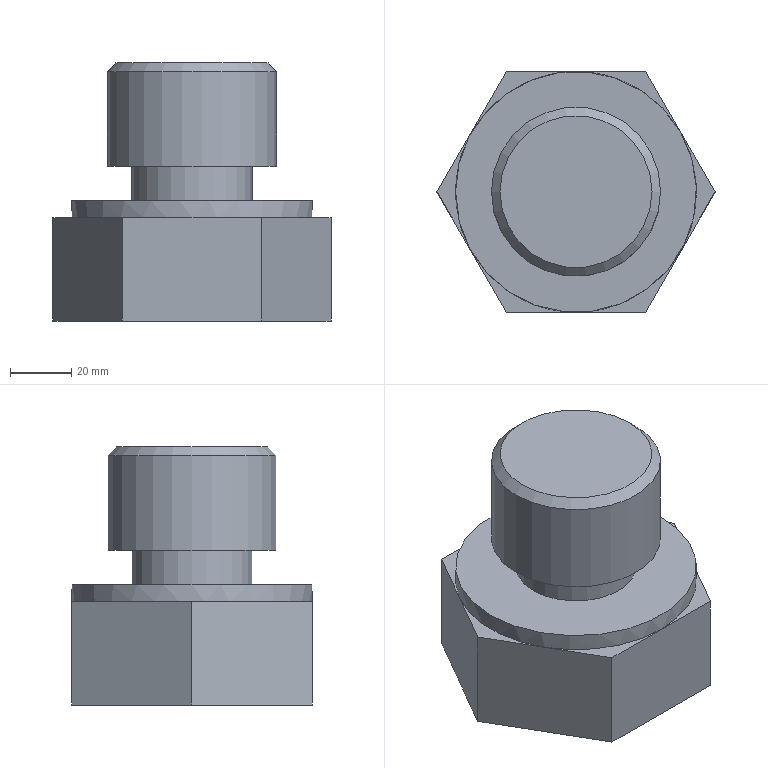Part | NX | features BOSS 2, CHAMFER 1, CYLINDER 1, DATUM_CSYS 1, Delete Body 1, EXTRUDE 1, LINKED_BODY 1, SCALE 1, SYMBOLIC_THREAD 1 | 1 solid | 20 faces | volume 302869 mm3 | plane 16 | cylinder 3 | cone 1 | commonest cylinder face diameters 39.375 x1 55.339 x1 78.75 x1